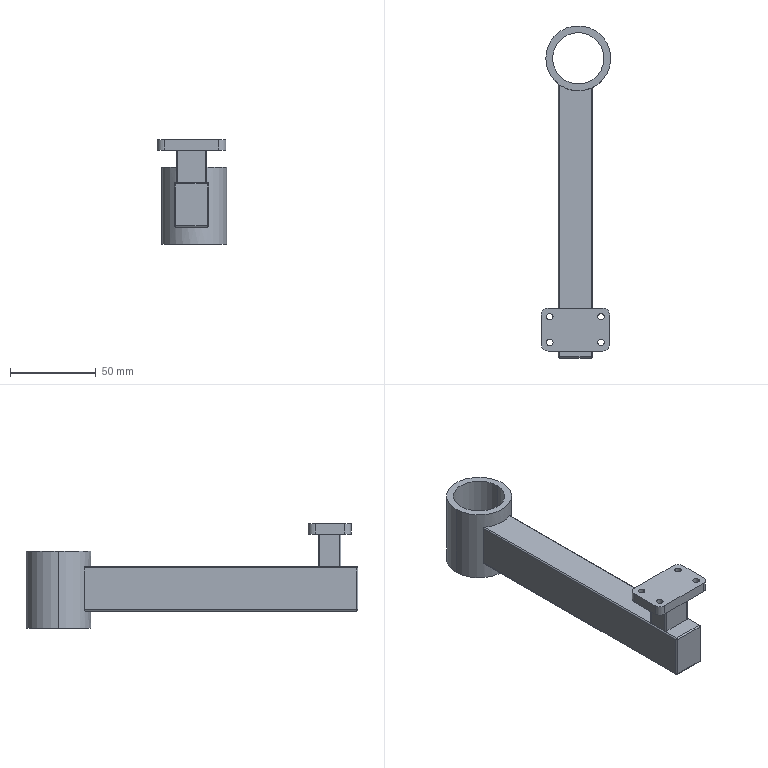Part | SolidWorks | features ICE 3, Extrusion 1, Fillet 1 | 1 solid | 49 faces | box 40.662 x 194 x 61 mm | volume 110850 mm3 | cylinder 28 | plane 17 | sphere 4 | commonest cylinder face diameters 1.6 x12 3.8 x8 8 x4 30 x2 38 x2
STEP:
#1=CARTESIAN_POINT('',(16.662,158.5,-10.));
#2=VERTEX_POINT('',#1);
#3=CARTESIAN_POINT('',(-13.338,158.5,-10.));
#4=VERTEX_POINT('',#3);
#5=CARTESIAN_POINT('',(1.662,158.5,-10.));
#6=DIRECTION('',(0.,0.,-1.));
#7=DIRECTION('',(-1.,0.,0.));
#8=AXIS2_PLACEMENT_3D('',#5,#6,#7);
#9=CIRCLE('',#8,15.);
#10=EDGE_CURVE('',#2,#4,#9,.T.);
#11=ORIENTED_EDGE('',*,*,#10,.F.);
#12=CARTESIAN_POINT('',(16.662,158.5,-55.));
#13=VERTEX_POINT('',#12);
#14=CARTESIAN_POINT('',(16.662,158.5,-10.));
#15=DIRECTION('',(0.,0.,-1.));
#16=VECTOR('',#15,1000.);
#17=LINE('',#14,#16);
#18=EDGE_CURVE('',#2,#13,#17,.T.);
#19=ORIENTED_EDGE('',*,*,#18,.T.);
#20=CARTESIAN_POINT('',(-13.338,158.5,-55.));
#21=VERTEX_POINT('',#20);
#22=CARTESIAN_POINT('',(1.662,158.5,-55.));
#23=DIRECTION('',(0.,0.,-1.));
#24=DIRECTION('',(-1.,0.,0.));
#25=AXIS2_PLACEMENT_3D('',#22,#23,#24);
#26=CIRCLE('',#25,15.);
#27=EDGE_CURVE('',#13,#21,#26,.T.);
#28=ORIENTED_EDGE('',*,*,#27,.T.);
#29=CARTESIAN_POINT('',(-13.338,158.5,-10.));
#30=DIRECTION('',(0.,0.,-1.));
#31=VECTOR('',#30,1000.);
#32=LINE('',#29,#31);
#33=EDGE_CURVE('',#4,#21,#32,.T.);
#34=ORIENTED_EDGE('',*,*,#33,.F.);
#35=EDGE_LOOP('',(#11,#19,#28,#34));
#36=FACE_OUTER_BOUND('',#35,.T.);
#37=CARTESIAN_POINT('',(1.662,158.5,-10.));
#38=DIRECTION('',(0.,0.,-1.));
#39=DIRECTION('',(-1.,0.,0.));
#40=AXIS2_PLACEMENT_3D('',#37,#38,#39);
#41=CYLINDRICAL_SURFACE('',#40,15.);
#42=ADVANCED_FACE('',(#36),#41,.F.);
#43=CARTESIAN_POINT('',(-17.338,158.5,-10.));
#44=VERTEX_POINT('',#43);
#45=CARTESIAN_POINT('',(20.662,158.5,-10.));
#46=VERTEX_POINT('',#45);
#47=CARTESIAN_POINT('',(1.662,158.5,-10.));
#48=DIRECTION('',(0.,0.,-1.));
#49=DIRECTION('',(-1.,0.,0.));
#50=AXIS2_PLACEMENT_3D('',#47,#48,#49);
#51=CIRCLE('',#50,19.);
#52=EDGE_CURVE('',#44,#46,#51,.T.);
#53=ORIENTED_EDGE('',*,*,#52,.T.);
#54=CARTESIAN_POINT('',(20.662,158.5,-55.));
#55=VERTEX_POINT('',#54);
#56=CARTESIAN_POINT('',(20.662,158.5,-10.));
#57=DIRECTION('',(0.,0.,-1.));
#58=VECTOR('',#57,1000.);
#59=LINE('',#56,#58);
#60=EDGE_CURVE('',#46,#55,#59,.T.);
#61=ORIENTED_EDGE('',*,*,#60,.T.);
#62=CARTESIAN_POINT('',(-17.338,158.5,-55.));
#63=VERTEX_POINT('',#62);
#64=CARTESIAN_POINT('',(1.662,158.5,-55.));
#65=DIRECTION('',(0.,0.,-1.));
#66=DIRECTION('',(-1.,0.,0.));
#67=AXIS2_PLACEMENT_3D('',#64,#65,#66);
#68=CIRCLE('',#67,19.);
#69=EDGE_CURVE('',#63,#55,#68,.T.);
#70=ORIENTED_EDGE('',*,*,#69,.F.);
#71=CARTESIAN_POINT('',(-17.338,158.5,-10.));
#72=DIRECTION('',(0.,0.,-1.));
#73=VECTOR('',#72,1000.);
#74=LINE('',#71,#73);
#75=EDGE_CURVE('',#44,#63,#74,.T.);
#76=ORIENTED_EDGE('',*,*,#75,.F.);
#77=EDGE_LOOP('',(#53,#61,#70,#76));
#78=FACE_OUTER_BOUND('',#77,.T.);
#79=CARTESIAN_POINT('',(1.662,158.5,-10.));
#80=DIRECTION('',(0.,0.,-1.));
#81=DIRECTION('',(-1.,0.,0.));
#82=AXIS2_PLACEMENT_3D('',#79,#80,#81);
#83=CYLINDRICAL_SURFACE('',#82,19.);
#84=ADVANCED_FACE('',(#78),#83,.T.);
#85=CARTESIAN_POINT('',(-16.9,-7.5,6.));
#86=VERTEX_POINT('',#85);
#87=CARTESIAN_POINT('',(-13.1,-7.5,6.));
#88=VERTEX_POINT('',#87);
#89=CARTESIAN_POINT('',(-15.,-7.5,6.));
#90=DIRECTION('',(0.,0.,1.));
#91=DIRECTION('',(1.,0.,0.));
#92=AXIS2_PLACEMENT_3D('',#89,#90,#91);
#93=CIRCLE('',#92,1.9);
#94=EDGE_CURVE('',#86,#88,#93,.T.);
#95=ORIENTED_EDGE('',*,*,#94,.T.);
#96=CARTESIAN_POINT('',(-13.1,-7.5,0.));
#97=VERTEX_POINT('',#96);
#98=CARTESIAN_POINT('',(-13.1,-7.5,6.));
#99=DIRECTION('',(0.,0.,-1.));
#100=VECTOR('',#99,1000.);
#101=LINE('',#98,#100);
#102=EDGE_CURVE('',#88,#97,#101,.T.);
#103=ORIENTED_EDGE('',*,*,#102,.T.);
#104=CARTESIAN_POINT('',(-16.9,-7.5,0.));
#105=VERTEX_POINT('',#104);
#106=CARTESIAN_POINT('',(-15.,-7.5,0.));
#107=DIRECTION('',(0.,0.,1.));
#108=DIRECTION('',(1.,0.,0.));
#109=AXIS2_PLACEMENT_3D('',#106,#107,#108);
#110=CIRCLE('',#109,1.9);
#111=EDGE_CURVE('',#105,#97,#110,.T.);
#112=ORIENTED_EDGE('',*,*,#111,.F.);
#113=CARTESIAN_POINT('',(-16.9,-7.5,6.));
#114=DIRECTION('',(0.,0.,-1.));
#115=VECTOR('',#114,1000.);
#116=LINE('',#113,#115);
#117=EDGE_CURVE('',#86,#105,#116,.T.);
#118=ORIENTED_EDGE('',*,*,#117,.F.);
#119=EDGE_LOOP('',(#95,#103,#112,#118));
#120=FACE_OUTER_BOUND('',#119,.T.);
#121=CARTESIAN_POINT('',(-15.,-7.5,6.));
#122=DIRECTION('',(0.,0.,-1.));
#123=DIRECTION('',(-1.,0.,0.));
#124=AXIS2_PLACEMENT_3D('',#121,#122,#123);
#125=CYLINDRICAL_SURFACE('',#124,1.9);
#126=ADVANCED_FACE('',(#120),#125,.F.);
#127=CARTESIAN_POINT('',(13.1,-7.5,6.));
#128=VERTEX_POINT('',#127);
#129=CARTESIAN_POINT('',(16.9,-7.5,6.));
#130=VERTEX_POINT('',#129);
#131=CARTESIAN_POINT('',(15.,-7.5,6.));
#132=DIRECTION('',(0.,0.,1.));
#133=DIRECTION('',(1.,0.,0.));
#134=AXIS2_PLACEMENT_3D('',#131,#132,#133);
#135=CIRCLE('',#134,1.9);
#136=EDGE_CURVE('',#128,#130,#135,.T.);
#137=ORIENTED_EDGE('',*,*,#136,.T.);
#138=CARTESIAN_POINT('',(16.9,-7.5,0.));
#139=VERTEX_POINT('',#138);
#140=CARTESIAN_POINT('',(16.9,-7.5,6.));
#141=DIRECTION('',(0.,0.,-1.));
#142=VECTOR('',#141,1000.);
#143=LINE('',#140,#142);
#144=EDGE_CURVE('',#130,#139,#143,.T.);
#145=ORIENTED_EDGE('',*,*,#144,.T.);
#146=CARTESIAN_POINT('',(13.1,-7.5,0.));
#147=VERTEX_POINT('',#146);
#148=CARTESIAN_POINT('',(15.,-7.5,0.));
#149=DIRECTION('',(0.,0.,1.));
#150=DIRECTION('',(1.,0.,0.));
#151=AXIS2_PLACEMENT_3D('',#148,#149,#150);
#152=CIRCLE('',#151,1.9);
#153=EDGE_CURVE('',#147,#139,#152,.T.);
#154=ORIENTED_EDGE('',*,*,#153,.F.);
#155=CARTESIAN_POINT('',(13.1,-7.5,6.));
#156=DIRECTION('',(0.,0.,-1.));
#157=VECTOR('',#156,1000.);
#158=LINE('',#155,#157);
#159=EDGE_CURVE('',#128,#147,#158,.T.);
#160=ORIENTED_EDGE('',*,*,#159,.F.);
#161=EDGE_LOOP('',(#137,#145,#154,#160));
#162=FACE_OUTER_BOUND('',#161,.T.);
#163=CARTESIAN_POINT('',(15.,-7.5,6.));
#164=DIRECTION('',(0.,0.,-1.));
#165=DIRECTION('',(-1.,0.,0.));
#166=AXIS2_PLACEMENT_3D('',#163,#164,#165);
#167=CYLINDRICAL_SURFACE('',#166,1.9);
#168=ADVANCED_FACE('',(#162),#167,.F.);
#169=CARTESIAN_POINT('',(13.1,7.5,6.));
#170=VERTEX_POINT('',#169);
#171=CARTESIAN_POINT('',(16.9,7.5,6.));
#172=VERTEX_POINT('',#171);
#173=CARTESIAN_POINT('',(15.,7.5,6.));
#174=DIRECTION('',(0.,0.,1.));
#175=DIRECTION('',(1.,0.,0.));
#176=AXIS2_PLACEMENT_3D('',#173,#174,#175);
#177=CIRCLE('',#176,1.9);
#178=EDGE_CURVE('',#170,#172,#177,.T.);
#179=ORIENTED_EDGE('',*,*,#178,.T.);
#180=CARTESIAN_POINT('',(16.9,7.5,0.));
#181=VERTEX_POINT('',#180);
#182=CARTESIAN_POINT('',(16.9,7.5,6.));
#183=DIRECTION('',(0.,0.,-1.));
#184=VECTOR('',#183,1000.);
#185=LINE('',#182,#184);
#186=EDGE_CURVE('',#172,#181,#185,.T.);
#187=ORIENTED_EDGE('',*,*,#186,.T.);
#188=CARTESIAN_POINT('',(13.1,7.5,0.));
#189=VERTEX_POINT('',#188);
#190=CARTESIAN_POINT('',(15.,7.5,0.));
#191=DIRECTION('',(0.,0.,1.));
#192=DIRECTION('',(1.,0.,0.));
#193=AXIS2_PLACEMENT_3D('',#190,#191,#192);
#194=CIRCLE('',#193,1.9);
#195=EDGE_CURVE('',#189,#181,#194,.T.);
#196=ORIENTED_EDGE('',*,*,#195,.F.);
#197=CARTESIAN_POINT('',(13.1,7.5,6.));
#198=DIRECTION('',(0.,0.,-1.));
#199=VECTOR('',#198,1000.);
#200=LINE('',#197,#199);
#201=EDGE_CURVE('',#170,#189,#200,.T.);
#202=ORIENTED_EDGE('',*,*,#201,.F.);
#203=EDGE_LOOP('',(#179,#187,#196,#202));
#204=FACE_OUTER_BOUND('',#203,.T.);
#205=CARTESIAN_POINT('',(15.,7.5,6.));
#206=DIRECTION('',(0.,0.,-1.));
#207=DIRECTION('',(-1.,0.,0.));
#208=AXIS2_PLACEMENT_3D('',#205,#206,#207);
#209=CYLINDRICAL_SURFACE('',#208,1.9);
#210=ADVANCED_FACE('',(#204),#209,.F.);
#211=CARTESIAN_POINT('',(-16.9,7.5,6.));
#212=VERTEX_POINT('',#211);
#213=CARTESIAN_POINT('',(-13.1,7.5,6.));
#214=VERTEX_POINT('',#213);
#215=CARTESIAN_POINT('',(-15.,7.5,6.));
#216=DIRECTION('',(0.,0.,1.));
#217=DIRECTION('',(1.,0.,0.));
#218=AXIS2_PLACEMENT_3D('',#215,#216,#217);
#219=CIRCLE('',#218,1.9);
#220=EDGE_CURVE('',#212,#214,#219,.T.);
#221=ORIENTED_EDGE('',*,*,#220,.T.);
#222=CARTESIAN_POINT('',(-13.1,7.5,0.));
#223=VERTEX_POINT('',#222);
#224=CARTESIAN_POINT('',(-13.1,7.5,6.));
#225=DIRECTION('',(0.,0.,-1.));
#226=VECTOR('',#225,1000.);
#227=LINE('',#224,#226);
#228=EDGE_CURVE('',#214,#223,#227,.T.);
#229=ORIENTED_EDGE('',*,*,#228,.T.);
#230=CARTESIAN_POINT('',(-16.9,7.5,0.));
#231=VERTEX_POINT('',#230);
#232=CARTESIAN_POINT('',(-15.,7.5,0.));
#233=DIRECTION('',(0.,0.,1.));
#234=DIRECTION('',(1.,0.,0.));
#235=AXIS2_PLACEMENT_3D('',#232,#233,#234);
#236=CIRCLE('',#235,1.9);
#237=EDGE_CURVE('',#231,#223,#236,.T.);
#238=ORIENTED_EDGE('',*,*,#237,.F.);
#239=CARTESIAN_POINT('',(-16.9,7.5,6.));
#240=DIRECTION('',(0.,0.,-1.));
#241=VECTOR('',#240,1000.);
#242=LINE('',#239,#241);
#243=EDGE_CURVE('',#212,#231,#242,.T.);
#244=ORIENTED_EDGE('',*,*,#243,.F.);
#245=EDGE_LOOP('',(#221,#229,#238,#244));
#246=FACE_OUTER_BOUND('',#245,.T.);
#247=CARTESIAN_POINT('',(-15.,7.5,6.));
#248=DIRECTION('',(0.,0.,-1.));
#249=DIRECTION('',(-1.,0.,0.));
#250=AXIS2_PLACEMENT_3D('',#247,#248,#249);
#251=CYLINDRICAL_SURFACE('',#250,1.9);
#252=ADVANCED_FACE('',(#246),#251,.F.);
#253=ORIENTED_EDGE('',*,*,#111,.T.);
#254=CARTESIAN_POINT('',(-15.,-7.5,0.));
#255=DIRECTION('',(0.,0.,1.));
#256=DIRECTION('',(1.,0.,0.));
#257=AXIS2_PLACEMENT_3D('',#254,#255,#256);
#258=CIRCLE('',#257,1.9);
#259=EDGE_CURVE('',#97,#105,#258,.T.);
#260=ORIENTED_EDGE('',*,*,#259,.T.);
#261=EDGE_LOOP('',(#253,#260));
#262=FACE_BOUND('',#261,.T.);
#263=ORIENTED_EDGE('',*,*,#153,.T.);
#264=CARTESIAN_POINT('',(15.,-7.5,0.));
#265=DIRECTION('',(0.,0.,1.));
#266=DIRECTION('',(1.,0.,0.));
#267=AXIS2_PLACEMENT_3D('',#264,#265,#266);
#268=CIRCLE('',#267,1.9);
#269=EDGE_CURVE('',#139,#147,#268,.T.);
#270=ORIENTED_EDGE('',*,*,#269,.T.);
#271=EDGE_LOOP('',(#263,#270));
#272=FACE_BOUND('',#271,.T.);
#273=ORIENTED_EDGE('',*,*,#195,.T.);
#274=CARTESIAN_POINT('',(15.,7.5,0.));
#275=DIRECTION('',(0.,0.,1.));
#276=DIRECTION('',(1.,0.,0.));
#277=AXIS2_PLACEMENT_3D('',#274,#275,#276);
#278=CIRCLE('',#277,1.9);
#279=EDGE_CURVE('',#181,#189,#278,.T.);
#280=ORIENTED_EDGE('',*,*,#279,.T.);
#281=EDGE_LOOP('',(#273,#280));
#282=FACE_BOUND('',#281,.T.);
#283=ORIENTED_EDGE('',*,*,#237,.T.);
#284=CARTESIAN_POINT('',(-15.,7.5,0.));
#285=DIRECTION('',(0.,0.,1.));
#286=DIRECTION('',(1.,0.,0.));
#287=AXIS2_PLACEMENT_3D('',#284,#285,#286);
#288=CIRCLE('',#287,1.9);
#289=EDGE_CURVE('',#223,#231,#288,.T.);
#290=ORIENTED_EDGE('',*,*,#289,.T.);
#291=EDGE_LOOP('',(#283,#290));
#292=FACE_BOUND('',#291,.T.);
#293=CARTESIAN_POINT('',(-20.,-8.5,0.));
#294=VERTEX_POINT('',#293);
#295=CARTESIAN_POINT('',(-16.,-12.5,0.));
#296=VERTEX_POINT('',#295);
#297=CARTESIAN_POINT('',(-16.,-8.5,0.));
#298=DIRECTION('',(0.,0.,1.));
#299=DIRECTION('',(1.,0.,0.));
#300=AXIS2_PLACEMENT_3D('',#297,#298,#299);
#301=CIRCLE('',#300,4.);
#302=EDGE_CURVE('',#294,#296,#301,.T.);
#303=ORIENTED_EDGE('',*,*,#302,.F.);
#304=CARTESIAN_POINT('',(-20.,8.5,0.));
#305=VERTEX_POINT('',#304);
#306=CARTESIAN_POINT('',(-20.,8.5,0.));
#307=DIRECTION('',(0.,-1.,0.));
#308=VECTOR('',#307,1000.);
#309=LINE('',#306,#308);
#310=EDGE_CURVE('',#305,#294,#309,.T.);
#311=ORIENTED_EDGE('',*,*,#310,.F.);
#312=CARTESIAN_POINT('',(-16.,12.5,0.));
#313=VERTEX_POINT('',#312);
#314=CARTESIAN_POINT('',(-16.,8.5,0.));
#315=DIRECTION('',(0.,0.,1.));
#316=DIRECTION('',(1.,0.,0.));
#317=AXIS2_PLACEMENT_3D('',#314,#315,#316);
#318=CIRCLE('',#317,4.);
#319=EDGE_CURVE('',#313,#305,#318,.T.);
#320=ORIENTED_EDGE('',*,*,#319,.F.);
#321=CARTESIAN_POINT('',(16.,12.5,0.));
#322=VERTEX_POINT('',#321);
#323=CARTESIAN_POINT('',(-16.,12.5,0.));
#324=DIRECTION('',(-1.,0.,0.));
#325=VECTOR('',#324,1000.);
#326=LINE('',#323,#325);
#327=EDGE_CURVE('',#322,#313,#326,.T.);
#328=ORIENTED_EDGE('',*,*,#327,.F.);
#329=CARTESIAN_POINT('',(20.,8.5,0.));
#330=VERTEX_POINT('',#329);
#331=CARTESIAN_POINT('',(16.,8.5,0.));
#332=DIRECTION('',(0.,0.,1.));
#333=DIRECTION('',(-1.,0.,0.));
#334=AXIS2_PLACEMENT_3D('',#331,#332,#333);
#335=CIRCLE('',#334,4.);
#336=EDGE_CURVE('',#330,#322,#335,.T.);
#337=ORIENTED_EDGE('',*,*,#336,.F.);
#338=CARTESIAN_POINT('',(20.,-8.5,0.));
#339=VERTEX_POINT('',#338);
#340=CARTESIAN_POINT('',(20.,8.5,0.));
#341=DIRECTION('',(0.,1.,0.));
#342=VECTOR('',#341,1000.);
#343=LINE('',#340,#342);
#344=EDGE_CURVE('',#339,#330,#343,.T.);
#345=ORIENTED_EDGE('',*,*,#344,.F.);
#346=CARTESIAN_POINT('',(16.,-12.5,0.));
#347=VERTEX_POINT('',#346);
#348=CARTESIAN_POINT('',(16.,-8.5,0.));
#349=DIRECTION('',(0.,0.,1.));
#350=DIRECTION('',(1.,0.,0.));
#351=AXIS2_PLACEMENT_3D('',#348,#349,#350);
#352=CIRCLE('',#351,4.);
#353=EDGE_CURVE('',#347,#339,#352,.T.);
#354=ORIENTED_EDGE('',*,*,#353,.F.);
#355=CARTESIAN_POINT('',(-16.,-12.5,0.));
#356=DIRECTION('',(1.,0.,0.));
#357=VECTOR('',#356,1000.);
#358=LINE('',#355,#357);
#359=EDGE_CURVE('',#296,#347,#358,.T.);
#360=ORIENTED_EDGE('',*,*,#359,.F.);
#361=EDGE_LOOP('',(#303,#311,#320,#328,#337,#345,#354,#360));
#362=FACE_OUTER_BOUND('',#361,.T.);
#363=CARTESIAN_POINT('',(-9.,-5.7,0.));
#364=VERTEX_POINT('',#363);
#365=CARTESIAN_POINT('',(-9.,5.7,0.));
#366=VERTEX_POINT('',#365);
#367=CARTESIAN_POINT('',(-9.,6.5,0.));
#368=DIRECTION('',(0.,1.,0.));
#369=VECTOR('',#368,1000.);
#370=LINE('',#367,#369);
#371=EDGE_CURVE('',#364,#366,#370,.T.);
#372=ORIENTED_EDGE('',*,*,#371,.F.);
#373=CARTESIAN_POINT('',(-8.2,-6.5,0.));
#374=VERTEX_POINT('',#373);
#375=CARTESIAN_POINT('',(-8.2,-5.7,0.));
#376=DIRECTION('',(0.,0.,1.));
#377=DIRECTION('',(1.,0.,0.));
#378=AXIS2_PLACEMENT_3D('',#375,#376,#377);
#379=CIRCLE('',#378,0.8);
#380=EDGE_CURVE('',#364,#374,#379,.T.);
#381=ORIENTED_EDGE('',*,*,#380,.T.);
#382=CARTESIAN_POINT('',(8.2,-6.5,0.));
#383=VERTEX_POINT('',#382);
#384=CARTESIAN_POINT('',(9.,-6.5,0.));
#385=DIRECTION('',(-1.,0.,0.));
#386=VECTOR('',#385,1000.);
#387=LINE('',#384,#386);
#388=EDGE_CURVE('',#383,#374,#387,.T.);
#389=ORIENTED_EDGE('',*,*,#388,.F.);
#390=CARTESIAN_POINT('',(9.,-5.7,0.));
#391=VERTEX_POINT('',#390);
#392=CARTESIAN_POINT('',(8.2,-5.7,0.));
#393=DIRECTION('',(0.,0.,1.));
#394=DIRECTION('',(1.,0.,0.));
#395=AXIS2_PLACEMENT_3D('',#392,#393,#394);
#396=CIRCLE('',#395,0.8);
#397=EDGE_CURVE('',#383,#391,#396,.T.);
#398=ORIENTED_EDGE('',*,*,#397,.T.);
#399=CARTESIAN_POINT('',(9.,5.7,0.));
#400=VERTEX_POINT('',#399);
#401=CARTESIAN_POINT('',(9.,6.5,0.));
#402=DIRECTION('',(0.,-1.,0.));
#403=VECTOR('',#402,1000.);
#404=LINE('',#401,#403);
#405=EDGE_CURVE('',#400,#391,#404,.T.);
#406=ORIENTED_EDGE('',*,*,#405,.F.);
#407=CARTESIAN_POINT('',(8.2,6.5,0.));
#408=VERTEX_POINT('',#407);
#409=CARTESIAN_POINT('',(8.2,5.7,0.));
#410=DIRECTION('',(0.,0.,1.));
#411=DIRECTION('',(1.,0.,0.));
#412=AXIS2_PLACEMENT_3D('',#409,#410,#411);
#413=CIRCLE('',#412,0.8);
#414=EDGE_CURVE('',#400,#408,#413,.T.);
#415=ORIENTED_EDGE('',*,*,#414,.T.);
#416=CARTESIAN_POINT('',(-8.2,6.5,0.));
#417=VERTEX_POINT('',#416);
#418=CARTESIAN_POINT('',(9.,6.5,0.));
#419=DIRECTION('',(1.,0.,0.));
#420=VECTOR('',#419,1000.);
#421=LINE('',#418,#420);
#422=EDGE_CURVE('',#417,#408,#421,.T.);
#423=ORIENTED_EDGE('',*,*,#422,.F.);
#424=CARTESIAN_POINT('',(-8.2,5.7,0.));
#425=DIRECTION('',(0.,0.,1.));
#426=DIRECTION('',(1.,0.,0.));
#427=AXIS2_PLACEMENT_3D('',#424,#425,#426);
#428=CIRCLE('',#427,0.8);
#429=EDGE_CURVE('',#417,#366,#428,.T.);
#430=ORIENTED_EDGE('',*,*,#429,.T.);
#431=EDGE_LOOP('',(#372,#381,#389,#398,#406,#415,#423,#430));
#432=FACE_BOUND('',#431,.T.);
#433=CARTESIAN_POINT('',(-16.,-8.5,0.));
#434=DIRECTION('',(0.,0.,1.));
#435=DIRECTION('',(1.,0.,0.));
#436=AXIS2_PLACEMENT_3D('',#433,#434,#435);
#437=PLANE('',#436);
#438=ADVANCED_FACE('',(#262,#272,#282,#292,#362,#432),#437,.F.);
#439=ORIENTED_EDGE('',*,*,#136,.F.);
#440=CARTESIAN_POINT('',(15.,-7.5,6.));
#441=DIRECTION('',(0.,0.,1.));
#442=DIRECTION('',(1.,0.,0.));
#443=AXIS2_PLACEMENT_3D('',#440,#441,#442);
#444=CIRCLE('',#443,1.9);
#445=EDGE_CURVE('',#130,#128,#444,.T.);
#446=ORIENTED_EDGE('',*,*,#445,.F.);
#447=EDGE_LOOP('',(#439,#446));
#448=FACE_BOUND('',#447,.T.);
#449=ORIENTED_EDGE('',*,*,#220,.F.);
#450=CARTESIAN_POINT('',(-15.,7.5,6.));
#451=DIRECTION('',(0.,0.,1.));
#452=DIRECTION('',(1.,0.,0.));
#453=AXIS2_PLACEMENT_3D('',#450,#451,#452);
#454=CIRCLE('',#453,1.9);
#455=EDGE_CURVE('',#214,#212,#454,.T.);
#456=ORIENTED_EDGE('',*,*,#455,.F.);
#457=EDGE_LOOP('',(#449,#456));
#458=FACE_BOUND('',#457,.T.);
#459=CARTESIAN_POINT('',(-20.,-8.5,6.));
#460=VERTEX_POINT('',#459);
#461=CARTESIAN_POINT('',(-16.,-12.5,6.));
#462=VERTEX_POINT('',#461);
#463=CARTESIAN_POINT('',(-16.,-8.5,6.));
#464=DIRECTION('',(0.,0.,1.));
#465=DIRECTION('',(1.,0.,0.));
#466=AXIS2_PLACEMENT_3D('',#463,#464,#465);
#467=CIRCLE('',#466,4.);
#468=EDGE_CURVE('',#460,#462,#467,.T.);
#469=ORIENTED_EDGE('',*,*,#468,.T.);
#470=CARTESIAN_POINT('',(16.,-12.5,6.));
#471=VERTEX_POINT('',#470);
#472=CARTESIAN_POINT('',(-16.,-12.5,6.));
#473=DIRECTION('',(1.,0.,0.));
#474=VECTOR('',#473,1000.);
#475=LINE('',#472,#474);
#476=EDGE_CURVE('',#462,#471,#475,.T.);
#477=ORIENTED_EDGE('',*,*,#476,.T.);
#478=CARTESIAN_POINT('',(20.,-8.5,6.));
#479=VERTEX_POINT('',#478);
#480=CARTESIAN_POINT('',(16.,-8.5,6.));
#481=DIRECTION('',(0.,0.,1.));
#482=DIRECTION('',(1.,0.,0.));
#483=AXIS2_PLACEMENT_3D('',#480,#481,#482);
#484=CIRCLE('',#483,4.);
#485=EDGE_CURVE('',#471,#479,#484,.T.);
#486=ORIENTED_EDGE('',*,*,#485,.T.);
#487=CARTESIAN_POINT('',(20.,8.5,6.));
#488=VERTEX_POINT('',#487);
#489=CARTESIAN_POINT('',(20.,8.5,6.));
#490=DIRECTION('',(0.,1.,0.));
#491=VECTOR('',#490,1000.);
#492=LINE('',#489,#491);
#493=EDGE_CURVE('',#479,#488,#492,.T.);
#494=ORIENTED_EDGE('',*,*,#493,.T.);
#495=CARTESIAN_POINT('',(16.,12.5,6.));
#496=VERTEX_POINT('',#495);
#497=CARTESIAN_POINT('',(16.,8.5,6.));
#498=DIRECTION('',(0.,0.,1.));
#499=DIRECTION('',(-1.,0.,0.));
#500=AXIS2_PLACEMENT_3D('',#497,#498,#499);
#501=CIRCLE('',#500,4.);
#502=EDGE_CURVE('',#488,#496,#501,.T.);
#503=ORIENTED_EDGE('',*,*,#502,.T.);
#504=CARTESIAN_POINT('',(-16.,12.5,6.));
#505=VERTEX_POINT('',#504);
#506=CARTESIAN_POINT('',(-16.,12.5,6.));
#507=DIRECTION('',(-1.,0.,0.));
#508=VECTOR('',#507,1000.);
#509=LINE('',#506,#508);
#510=EDGE_CURVE('',#496,#505,#509,.T.);
#511=ORIENTED_EDGE('',*,*,#510,.T.);
#512=CARTESIAN_POINT('',(-20.,8.5,6.));
#513=VERTEX_POINT('',#512);
#514=CARTESIAN_POINT('',(-16.,8.5,6.));
#515=DIRECTION('',(0.,0.,1.));
#516=DIRECTION('',(1.,0.,0.));
#517=AXIS2_PLACEMENT_3D('',#514,#515,#516);
#518=CIRCLE('',#517,4.);
#519=EDGE_CURVE('',#505,#513,#518,.T.);
#520=ORIENTED_EDGE('',*,*,#519,.T.);
#521=CARTESIAN_POINT('',(-20.,8.5,6.));
#522=DIRECTION('',(0.,-1.,0.));
#523=VECTOR('',#522,1000.);
#524=LINE('',#521,#523);
#525=EDGE_CURVE('',#513,#460,#524,.T.);
#526=ORIENTED_EDGE('',*,*,#525,.T.);
#527=EDGE_LOOP('',(#469,#477,#486,#494,#503,#511,#520,#526));
#528=FACE_OUTER_BOUND('',#527,.T.);
#529=ORIENTED_EDGE('',*,*,#178,.F.);
#530=CARTESIAN_POINT('',(15.,7.5,6.));
#531=DIRECTION('',(0.,0.,1.));
#532=DIRECTION('',(1.,0.,0.));
#533=AXIS2_PLACEMENT_3D('',#530,#531,#532);
#534=CIRCLE('',#533,1.9);
#535=EDGE_CURVE('',#172,#170,#534,.T.);
#536=ORIENTED_EDGE('',*,*,#535,.F.);
#537=EDGE_LOOP('',(#529,#536));
#538=FACE_BOUND('',#537,.T.);
#539=ORIENTED_EDGE('',*,*,#94,.F.);
#540=CARTESIAN_POINT('',(-15.,-7.5,6.));
#541=DIRECTION('',(0.,0.,1.));
#542=DIRECTION('',(1.,0.,0.));
#543=AXIS2_PLACEMENT_3D('',#540,#541,#542);
#544=CIRCLE('',#543,1.9);
#545=EDGE_CURVE('',#88,#86,#544,.T.);
#546=ORIENTED_EDGE('',*,*,#545,.F.);
#547=EDGE_LOOP('',(#539,#546));
#548=FACE_BOUND('',#547,.T.);
#549=CARTESIAN_POINT('',(-16.,-8.5,6.));
#550=DIRECTION('',(0.,0.,1.));
#551=DIRECTION('',(1.,0.,0.));
#552=AXIS2_PLACEMENT_3D('',#549,#550,#551);
#553=PLANE('',#552);
#554=ADVANCED_FACE('',(#448,#458,#528,#538,#548),#553,.T.);
#555=ORIENTED_EDGE('',*,*,#302,.T.);
#556=CARTESIAN_POINT('',(-16.,-12.5,6.));
#557=DIRECTION('',(0.,0.,-1.));
#558=VECTOR('',#557,1000.);
#559=LINE('',#556,#558);
#560=EDGE_CURVE('',#462,#296,#559,.T.);
#561=ORIENTED_EDGE('',*,*,#560,.F.);
#562=ORIENTED_EDGE('',*,*,#468,.F.);
#563=CARTESIAN_POINT('',(-20.,-8.5,6.));
#564=DIRECTION('',(0.,0.,-1.));
#565=VECTOR('',#564,1000.);
#566=LINE('',#563,#565);
#567=EDGE_CURVE('',#460,#294,#566,.T.);
#568=ORIENTED_EDGE('',*,*,#567,.T.);
#569=EDGE_LOOP('',(#555,#561,#562,#568));
#570=FACE_OUTER_BOUND('',#569,.T.);
#571=CARTESIAN_POINT('',(-16.,-8.5,6.));
#572=DIRECTION('',(0.,0.,-1.));
#573=DIRECTION('',(-1.,0.,0.));
#574=AXIS2_PLACEMENT_3D('',#571,#572,#573);
#575=CYLINDRICAL_SURFACE('',#574,4.);
#576=ADVANCED_FACE('',(#570),#575,.T.);
#577=ORIENTED_EDGE('',*,*,#359,.T.);
#578=CARTESIAN_POINT('',(16.,-12.5,6.));
#579=DIRECTION('',(0.,0.,-1.));
#580=VECTOR('',#579,1000.);
#581=LINE('',#578,#580);
#582=EDGE_CURVE('',#471,#347,#581,.T.);
#583=ORIENTED_EDGE('',*,*,#582,.F.);
#584=ORIENTED_EDGE('',*,*,#476,.F.);
#585=ORIENTED_EDGE('',*,*,#560,.T.);
#586=EDGE_LOOP('',(#577,#583,#584,#585));
#587=FACE_OUTER_BOUND('',#586,.T.);
#588=CARTESIAN_POINT('',(-16.,-12.5,6.));
#589=DIRECTION('',(0.,1.,0.));
#590=DIRECTION('',(-1.,0.,0.));
#591=AXIS2_PLACEMENT_3D('',#588,#589,#590);
#592=PLANE('',#591);
#593=ADVANCED_FACE('',(#587),#592,.F.);
#594=ORIENTED_EDGE('',*,*,#353,.T.);
#595=CARTESIAN_POINT('',(20.,-8.5,6.));
#596=DIRECTION('',(0.,0.,-1.));
#597=VECTOR('',#596,1000.);
#598=LINE('',#595,#597);
#599=EDGE_CURVE('',#479,#339,#598,.T.);
#600=ORIENTED_EDGE('',*,*,#599,.F.);
#601=ORIENTED_EDGE('',*,*,#485,.F.);
#602=ORIENTED_EDGE('',*,*,#582,.T.);
#603=EDGE_LOOP('',(#594,#600,#601,#602));
#604=FACE_OUTER_BOUND('',#603,.T.);
#605=CARTESIAN_POINT('',(16.,-8.5,6.));
#606=DIRECTION('',(0.,0.,-1.));
#607=DIRECTION('',(-1.,0.,0.));
#608=AXIS2_PLACEMENT_3D('',#605,#606,#607);
#609=CYLINDRICAL_SURFACE('',#608,4.);
#610=ADVANCED_FACE('',(#604),#609,.T.);
#611=ORIENTED_EDGE('',*,*,#344,.T.);
#612=CARTESIAN_POINT('',(20.,8.5,6.));
#613=DIRECTION('',(0.,0.,-1.));
#614=VECTOR('',#613,1000.);
#615=LINE('',#612,#614);
#616=EDGE_CURVE('',#488,#330,#615,.T.);
#617=ORIENTED_EDGE('',*,*,#616,.F.);
#618=ORIENTED_EDGE('',*,*,#493,.F.);
#619=ORIENTED_EDGE('',*,*,#599,.T.);
#620=EDGE_LOOP('',(#611,#617,#618,#619));
#621=FACE_OUTER_BOUND('',#620,.T.);
#622=CARTESIAN_POINT('',(20.,8.5,6.));
#623=DIRECTION('',(-1.,0.,0.));
#624=DIRECTION('',(0.,-1.,0.));
#625=AXIS2_PLACEMENT_3D('',#622,#623,#624);
#626=PLANE('',#625);
#627=ADVANCED_FACE('',(#621),#626,.F.);
#628=ORIENTED_EDGE('',*,*,#336,.T.);
#629=CARTESIAN_POINT('',(16.,12.5,6.));
#630=DIRECTION('',(0.,0.,-1.));
#631=VECTOR('',#630,1000.);
#632=LINE('',#629,#631);
#633=EDGE_CURVE('',#496,#322,#632,.T.);
#634=ORIENTED_EDGE('',*,*,#633,.F.);
#635=ORIENTED_EDGE('',*,*,#502,.F.);
#636=ORIENTED_EDGE('',*,*,#616,.T.);
#637=EDGE_LOOP('',(#628,#634,#635,#636));
#638=FACE_OUTER_BOUND('',#637,.T.);
#639=CARTESIAN_POINT('',(16.,8.5,6.));
#640=DIRECTION('',(0.,0.,-1.));
#641=DIRECTION('',(-1.,0.,0.));
#642=AXIS2_PLACEMENT_3D('',#639,#640,#641);
#643=CYLINDRICAL_SURFACE('',#642,4.);
#644=ADVANCED_FACE('',(#638),#643,.T.);
#645=ORIENTED_EDGE('',*,*,#327,.T.);
#646=CARTESIAN_POINT('',(-16.,12.5,6.));
#647=DIRECTION('',(0.,0.,-1.));
#648=VECTOR('',#647,1000.);
#649=LINE('',#646,#648);
#650=EDGE_CURVE('',#505,#313,#649,.T.);
#651=ORIENTED_EDGE('',*,*,#650,.F.);
#652=ORIENTED_EDGE('',*,*,#510,.F.);
#653=ORIENTED_EDGE('',*,*,#633,.T.);
#654=EDGE_LOOP('',(#645,#651,#652,#653));
#655=FACE_OUTER_BOUND('',#654,.T.);
#656=CARTESIAN_POINT('',(-16.,12.5,6.));
#657=DIRECTION('',(0.,-1.,0.));
#658=DIRECTION('',(0.,0.,-1.));
#659=AXIS2_PLACEMENT_3D('',#656,#657,#658);
#660=PLANE('',#659);
#661=ADVANCED_FACE('',(#655),#660,.F.);
#662=ORIENTED_EDGE('',*,*,#319,.T.);
#663=CARTESIAN_POINT('',(-20.,8.5,6.));
#664=DIRECTION('',(0.,0.,-1.));
#665=VECTOR('',#664,1000.);
#666=LINE('',#663,#665);
#667=EDGE_CURVE('',#513,#305,#666,.T.);
#668=ORIENTED_EDGE('',*,*,#667,.F.);
#669=ORIENTED_EDGE('',*,*,#519,.F.);
#670=ORIENTED_EDGE('',*,*,#650,.T.);
#671=EDGE_LOOP('',(#662,#668,#669,#670));
#672=FACE_OUTER_BOUND('',#671,.T.);
#673=CARTESIAN_POINT('',(-16.,8.5,6.));
#674=DIRECTION('',(0.,0.,-1.));
#675=DIRECTION('',(-1.,0.,0.));
#676=AXIS2_PLACEMENT_3D('',#673,#674,#675);
#677=CYLINDRICAL_SURFACE('',#676,4.);
#678=ADVANCED_FACE('',(#672),#677,.T.);
#679=ORIENTED_EDGE('',*,*,#310,.T.);
#680=ORIENTED_EDGE('',*,*,#567,.F.);
#681=ORIENTED_EDGE('',*,*,#525,.F.);
#682=ORIENTED_EDGE('',*,*,#667,.T.);
#683=EDGE_LOOP('',(#679,#680,#681,#682));
#684=FACE_OUTER_BOUND('',#683,.T.);
#685=CARTESIAN_POINT('',(-20.,8.5,6.));
#686=DIRECTION('',(1.,0.,0.));
#687=DIRECTION('',(0.,1.,0.));
#688=AXIS2_PLACEMENT_3D('',#685,#686,#687);
#689=PLANE('',#688);
#690=ADVANCED_FACE('',(#684),#689,.F.);
#691=ORIENTED_EDGE('',*,*,#228,.F.);
#692=ORIENTED_EDGE('',*,*,#455,.T.);
#693=ORIENTED_EDGE('',*,*,#243,.T.);
#694=ORIENTED_EDGE('',*,*,#289,.F.);
#695=EDGE_LOOP('',(#691,#692,#693,#694));
#696=FACE_OUTER_BOUND('',#695,.T.);
#697=CARTESIAN_POINT('',(-15.,7.5,6.));
#698=DIRECTION('',(0.,0.,-1.));
#699=DIRECTION('',(-1.,0.,0.));
#700=AXIS2_PLACEMENT_3D('',#697,#698,#699);
#701=CYLINDRICAL_SURFACE('',#700,1.9);
#702=ADVANCED_FACE('',(#696),#701,.F.);
#703=ORIENTED_EDGE('',*,*,#186,.F.);
#704=ORIENTED_EDGE('',*,*,#535,.T.);
#705=ORIENTED_EDGE('',*,*,#201,.T.);
#706=ORIENTED_EDGE('',*,*,#279,.F.);
#707=EDGE_LOOP('',(#703,#704,#705,#706));
#708=FACE_OUTER_BOUND('',#707,.T.);
#709=CARTESIAN_POINT('',(15.,7.5,6.));
#710=DIRECTION('',(0.,0.,-1.));
#711=DIRECTION('',(-1.,0.,0.));
#712=AXIS2_PLACEMENT_3D('',#709,#710,#711);
#713=CYLINDRICAL_SURFACE('',#712,1.9);
#714=ADVANCED_FACE('',(#708),#713,.F.);
#715=ORIENTED_EDGE('',*,*,#144,.F.);
#716=ORIENTED_EDGE('',*,*,#445,.T.);
#717=ORIENTED_EDGE('',*,*,#159,.T.);
#718=ORIENTED_EDGE('',*,*,#269,.F.);
#719=EDGE_LOOP('',(#715,#716,#717,#718));
#720=FACE_OUTER_BOUND('',#719,.T.);
#721=CARTESIAN_POINT('',(15.,-7.5,6.));
#722=DIRECTION('',(0.,0.,-1.));
#723=DIRECTION('',(-1.,0.,0.));
#724=AXIS2_PLACEMENT_3D('',#721,#722,#723);
#725=CYLINDRICAL_SURFACE('',#724,1.9);
#726=ADVANCED_FACE('',(#720),#725,.F.);
#727=ORIENTED_EDGE('',*,*,#102,.F.);
#728=ORIENTED_EDGE('',*,*,#545,.T.);
#729=ORIENTED_EDGE('',*,*,#117,.T.);
#730=ORIENTED_EDGE('',*,*,#259,.F.);
#731=EDGE_LOOP('',(#727,#728,#729,#730));
#732=FACE_OUTER_BOUND('',#731,.T.);
#733=CARTESIAN_POINT('',(-15.,-7.5,6.));
#734=DIRECTION('',(0.,0.,-1.));
#735=DIRECTION('',(-1.,0.,0.));
#736=AXIS2_PLACEMENT_3D('',#733,#734,#735);
#737=CYLINDRICAL_SURFACE('',#736,1.9);
#738=ADVANCED_FACE('',(#732),#737,.F.);
#739=CARTESIAN_POINT('',(-9.,5.7,-19.));
#740=VERTEX_POINT('',#739);
#741=CARTESIAN_POINT('',(-9.,-5.7,-19.));
#742=VERTEX_POINT('',#741);
#743=CARTESIAN_POINT('',(-9.,6.5,-19.));
#744=DIRECTION('',(0.,-1.,0.));
#745=VECTOR('',#744,1000.);
#746=LINE('',#743,#745);
#747=EDGE_CURVE('',#740,#742,#746,.T.);
#748=ORIENTED_EDGE('',*,*,#747,.T.);
#749=CARTESIAN_POINT('',(-9.,-5.7,-32.));
#750=DIRECTION('',(0.,0.,1.));
#751=VECTOR('',#750,1000.);
#752=LINE('',#749,#751);
#753=EDGE_CURVE('',#742,#364,#752,.T.);
#754=ORIENTED_EDGE('',*,*,#753,.T.);
#755=ORIENTED_EDGE('',*,*,#371,.T.);
#756=CARTESIAN_POINT('',(-9.,5.7,-32.));
#757=DIRECTION('',(0.,0.,-1.));
#758=VECTOR('',#757,1000.);
#759=LINE('',#756,#758);
#760=EDGE_CURVE('',#366,#740,#759,.T.);
#761=ORIENTED_EDGE('',*,*,#760,.T.);
#762=EDGE_LOOP('',(#748,#754,#755,#761));
#763=FACE_OUTER_BOUND('',#762,.T.);
#764=CARTESIAN_POINT('',(-9.,6.5,-32.));
#765=DIRECTION('',(1.,0.,0.));
#766=DIRECTION('',(0.,0.,-1.));
#767=AXIS2_PLACEMENT_3D('',#764,#765,#766);
#768=PLANE('',#767);
#769=ADVANCED_FACE('',(#763),#768,.F.);
#770=ORIENTED_EDGE('',*,*,#422,.T.);
#771=CARTESIAN_POINT('',(8.2,6.5,-19.));
#772=VERTEX_POINT('',#771);
#773=CARTESIAN_POINT('',(8.2,6.5,-32.));
#774=DIRECTION('',(0.,0.,-1.));
#775=VECTOR('',#774,1000.);
#776=LINE('',#773,#775);
#777=EDGE_CURVE('',#408,#772,#776,.T.);
#778=ORIENTED_EDGE('',*,*,#777,.T.);
#779=CARTESIAN_POINT('',(-8.2,6.5,-19.));
#780=VERTEX_POINT('',#779);
#781=CARTESIAN_POINT('',(9.,6.5,-19.));
#782=DIRECTION('',(-1.,0.,0.));
#783=VECTOR('',#782,1000.);
#784=LINE('',#781,#783);
#785=EDGE_CURVE('',#772,#780,#784,.T.);
#786=ORIENTED_EDGE('',*,*,#785,.T.);
#787=CARTESIAN_POINT('',(-8.2,6.5,-32.));
#788=DIRECTION('',(0.,0.,1.));
#789=VECTOR('',#788,1000.);
#790=LINE('',#787,#789);
#791=EDGE_CURVE('',#780,#417,#790,.T.);
#792=ORIENTED_EDGE('',*,*,#791,.T.);
#793=EDGE_LOOP('',(#770,#778,#786,#792));
#794=FACE_OUTER_BOUND('',#793,.T.);
#795=CARTESIAN_POINT('',(9.,6.5,-32.));
#796=DIRECTION('',(0.,-1.,0.));
#797=DIRECTION('',(0.,0.,-1.));
#798=AXIS2_PLACEMENT_3D('',#795,#796,#797);
#799=PLANE('',#798);
#800=ADVANCED_FACE('',(#794),#799,.F.);
#801=CARTESIAN_POINT('',(9.,-5.7,-19.));
#802=VERTEX_POINT('',#801);
#803=CARTESIAN_POINT('',(9.,5.7,-19.));
#804=VERTEX_POINT('',#803);
#805=CARTESIAN_POINT('',(9.,6.5,-19.));
#806=DIRECTION('',(0.,1.,0.));
#807=VECTOR('',#806,1000.);
#808=LINE('',#805,#807);
#809=EDGE_CURVE('',#802,#804,#808,.T.);
#810=ORIENTED_EDGE('',*,*,#809,.T.);
#811=CARTESIAN_POINT('',(9.,5.7,-32.));
#812=DIRECTION('',(0.,0.,1.));
#813=VECTOR('',#812,1000.);
#814=LINE('',#811,#813);
#815=EDGE_CURVE('',#804,#400,#814,.T.);
#816=ORIENTED_EDGE('',*,*,#815,.T.);
#817=ORIENTED_EDGE('',*,*,#405,.T.);
#818=CARTESIAN_POINT('',(9.,-5.7,-32.));
#819=DIRECTION('',(0.,0.,-1.));
#820=VECTOR('',#819,1000.);
#821=LINE('',#818,#820);
#822=EDGE_CURVE('',#391,#802,#821,.T.);
#823=ORIENTED_EDGE('',*,*,#822,.T.);
#824=EDGE_LOOP('',(#810,#816,#817,#823));
#825=FACE_OUTER_BOUND('',#824,.T.);
#826=CARTESIAN_POINT('',(9.,6.5,-32.));
#827=DIRECTION('',(-1.,0.,0.));
#828=DIRECTION('',(0.,0.,1.));
#829=AXIS2_PLACEMENT_3D('',#826,#827,#828);
#830=PLANE('',#829);
#831=ADVANCED_FACE('',(#825),#830,.F.);
#832=CARTESIAN_POINT('',(-8.2,-6.5,-19.));
#833=VERTEX_POINT('',#832);
#834=CARTESIAN_POINT('',(8.2,-6.5,-19.));
#835=VERTEX_POINT('',#834);
#836=CARTESIAN_POINT('',(9.,-6.5,-19.));
#837=DIRECTION('',(1.,0.,0.));
#838=VECTOR('',#837,1000.);
#839=LINE('',#836,#838);
#840=EDGE_CURVE('',#833,#835,#839,.T.);
#841=ORIENTED_EDGE('',*,*,#840,.T.);
#842=CARTESIAN_POINT('',(8.2,-6.5,-32.));
#843=DIRECTION('',(0.,0.,1.));
#844=VECTOR('',#843,1000.);
#845=LINE('',#842,#844);
#846=EDGE_CURVE('',#835,#383,#845,.T.);
#847=ORIENTED_EDGE('',*,*,#846,.T.);
#848=ORIENTED_EDGE('',*,*,#388,.T.);
#849=CARTESIAN_POINT('',(-8.2,-6.5,-32.));
#850=DIRECTION('',(0.,0.,-1.));
#851=VECTOR('',#850,1000.);
#852=LINE('',#849,#851);
#853=EDGE_CURVE('',#374,#833,#852,.T.);
#854=ORIENTED_EDGE('',*,*,#853,.T.);
#855=EDGE_LOOP('',(#841,#847,#848,#854));
#856=FACE_OUTER_BOUND('',#855,.T.);
#857=CARTESIAN_POINT('',(9.,-6.5,-32.));
#858=DIRECTION('',(0.,1.,0.));
#859=DIRECTION('',(0.,0.,1.));
#860=AXIS2_PLACEMENT_3D('',#857,#858,#859);
#861=PLANE('',#860);
#862=ADVANCED_FACE('',(#856),#861,.F.);
#863=CARTESIAN_POINT('',(-9.2,-15.7,-19.));
#864=VERTEX_POINT('',#863);
#865=CARTESIAN_POINT('',(9.2,-15.7,-19.));
#866=VERTEX_POINT('',#865);
#867=CARTESIAN_POINT('',(-10.,-15.7,-19.));
#868=DIRECTION('',(1.,0.,0.));
#869=VECTOR('',#868,1000.);
#870=LINE('',#867,#869);
#871=EDGE_CURVE('',#864,#866,#870,.T.);
#872=ORIENTED_EDGE('',*,*,#871,.T.);
#873=CARTESIAN_POINT('',(9.2,141.059,-19.));
#874=VERTEX_POINT('',#873);
#875=CARTESIAN_POINT('',(9.2,143.5,-19.));
#876=DIRECTION('',(0.,1.,0.));
#877=VECTOR('',#876,1000.);
#878=LINE('',#875,#877);
#879=EDGE_CURVE('',#866,#874,#878,.T.);
#880=ORIENTED_EDGE('',*,*,#879,.T.);
#881=CARTESIAN_POINT('',(-9.2,142.911,-19.));
#882=VERTEX_POINT('',#881);
#883=CARTESIAN_POINT('',(1.662,158.5,-19.));
#884=DIRECTION('',(0.,0.,1.));
#885=DIRECTION('',(1.,0.,0.));
#886=AXIS2_PLACEMENT_3D('',#883,#884,#885);
#887=CIRCLE('',#886,19.);
#888=EDGE_CURVE('',#882,#874,#887,.T.);
#889=ORIENTED_EDGE('',*,*,#888,.F.);
#890=CARTESIAN_POINT('',(-9.2,143.5,-19.));
#891=DIRECTION('',(0.,-1.,0.));
#892=VECTOR('',#891,1000.);
#893=LINE('',#890,#892);
#894=EDGE_CURVE('',#882,#864,#893,.T.);
#895=ORIENTED_EDGE('',*,*,#894,.T.);
#896=EDGE_LOOP('',(#872,#880,#889,#895));
#897=FACE_OUTER_BOUND('',#896,.T.);
#898=ORIENTED_EDGE('',*,*,#747,.F.);
#899=CARTESIAN_POINT('',(-8.2,5.7,-19.));
#900=DIRECTION('',(0.,0.,-1.));
#901=DIRECTION('',(1.,0.,0.));
#902=AXIS2_PLACEMENT_3D('',#899,#900,#901);
#903=CIRCLE('',#902,0.8);
#904=EDGE_CURVE('',#740,#780,#903,.T.);
#905=ORIENTED_EDGE('',*,*,#904,.T.);
#906=ORIENTED_EDGE('',*,*,#785,.F.);
#907=CARTESIAN_POINT('',(8.2,5.7,-19.));
#908=DIRECTION('',(0.,0.,-1.));
#909=DIRECTION('',(1.,0.,0.));
#910=AXIS2_PLACEMENT_3D('',#907,#908,#909);
#911=CIRCLE('',#910,0.8);
#912=EDGE_CURVE('',#772,#804,#911,.T.);
#913=ORIENTED_EDGE('',*,*,#912,.T.);
#914=ORIENTED_EDGE('',*,*,#809,.F.);
#915=CARTESIAN_POINT('',(8.2,-5.7,-19.));
#916=DIRECTION('',(0.,0.,-1.));
#917=DIRECTION('',(1.,0.,0.));
#918=AXIS2_PLACEMENT_3D('',#915,#916,#917);
#919=CIRCLE('',#918,0.8);
#920=EDGE_CURVE('',#802,#835,#919,.T.);
#921=ORIENTED_EDGE('',*,*,#920,.T.);
#922=ORIENTED_EDGE('',*,*,#840,.F.);
#923=CARTESIAN_POINT('',(-8.2,-5.7,-19.));
#924=DIRECTION('',(0.,0.,-1.));
#925=DIRECTION('',(1.,0.,0.));
#926=AXIS2_PLACEMENT_3D('',#923,#924,#925);
#927=CIRCLE('',#926,0.8);
#928=EDGE_CURVE('',#833,#742,#927,.T.);
#929=ORIENTED_EDGE('',*,*,#928,.T.);
#930=EDGE_LOOP('',(#898,#905,#906,#913,#914,#921,#922,#929));
#931=FACE_BOUND('',#930,.T.);
#932=CARTESIAN_POINT('',(-10.,143.5,-19.));
#933=DIRECTION('',(0.,0.,1.));
#934=DIRECTION('',(1.,0.,0.));
#935=AXIS2_PLACEMENT_3D('',#932,#933,#934);
#936=PLANE('',#935);
#937=ADVANCED_FACE('',(#897,#931),#936,.T.);
#938=CARTESIAN_POINT('',(10.,141.427,-19.8));
#939=VERTEX_POINT('',#938);
#940=CARTESIAN_POINT('',(10.,141.427,-44.2));
#941=VERTEX_POINT('',#940);
#942=CARTESIAN_POINT('',(10.,141.427,-10.));
#943=DIRECTION('',(0.,0.,-1.));
#944=VECTOR('',#943,1000.);
#945=LINE('',#942,#944);
#946=EDGE_CURVE('',#939,#941,#945,.T.);
#947=ORIENTED_EDGE('',*,*,#946,.F.);
#948=CARTESIAN_POINT('',(10.,-15.7,-19.8));
#949=VERTEX_POINT('',#948);
#950=CARTESIAN_POINT('',(10.,143.5,-19.8));
#951=DIRECTION('',(0.,-1.,0.));
#952=VECTOR('',#951,1000.);
#953=LINE('',#950,#952);
#954=EDGE_CURVE('',#939,#949,#953,.T.);
#955=ORIENTED_EDGE('',*,*,#954,.T.);
#956=CARTESIAN_POINT('',(10.,-15.7,-44.2));
#957=VERTEX_POINT('',#956);
#958=CARTESIAN_POINT('',(10.,-15.7,-19.));
#959=DIRECTION('',(0.,0.,-1.));
#960=VECTOR('',#959,1000.);
#961=LINE('',#958,#960);
#962=EDGE_CURVE('',#949,#957,#961,.T.);
#963=ORIENTED_EDGE('',*,*,#962,.T.);
#964=CARTESIAN_POINT('',(10.,143.5,-44.2));
#965=DIRECTION('',(0.,1.,0.));
#966=VECTOR('',#965,1000.);
#967=LINE('',#964,#966);
#968=EDGE_CURVE('',#957,#941,#967,.T.);
#969=ORIENTED_EDGE('',*,*,#968,.T.);
#970=EDGE_LOOP('',(#947,#955,#963,#969));
#971=FACE_OUTER_BOUND('',#970,.T.);
#972=CARTESIAN_POINT('',(10.,143.5,-19.));
#973=DIRECTION('',(1.,0.,0.));
#974=DIRECTION('',(0.,0.,-1.));
#975=AXIS2_PLACEMENT_3D('',#972,#973,#974);
#976=PLANE('',#975);
#977=ADVANCED_FACE('',(#971),#976,.T.);
#978=CARTESIAN_POINT('',(9.2,141.059,-45.));
#979=VERTEX_POINT('',#978);
#980=CARTESIAN_POINT('',(-9.2,142.911,-45.));
#981=VERTEX_POINT('',#980);
#982=CARTESIAN_POINT('',(1.662,158.5,-45.));
#983=DIRECTION('',(0.,0.,-1.));
#984=DIRECTION('',(-1.,0.,0.));
#985=AXIS2_PLACEMENT_3D('',#982,#983,#984);
#986=CIRCLE('',#985,19.);
#987=EDGE_CURVE('',#979,#981,#986,.T.);
#988=ORIENTED_EDGE('',*,*,#987,.F.);
#989=CARTESIAN_POINT('',(9.2,-15.7,-45.));
#990=VERTEX_POINT('',#989);
#991=CARTESIAN_POINT('',(9.2,143.5,-45.));
#992=DIRECTION('',(0.,-1.,0.));
#993=VECTOR('',#992,1000.);
#994=LINE('',#991,#993);
#995=EDGE_CURVE('',#979,#990,#994,.T.);
#996=ORIENTED_EDGE('',*,*,#995,.T.);
#997=CARTESIAN_POINT('',(-9.2,-15.7,-45.));
#998=VERTEX_POINT('',#997);
#999=CARTESIAN_POINT('',(-10.,-15.7,-45.));
#1000=DIRECTION('',(-1.,0.,0.));
#1001=VECTOR('',#1000,1000.);
#1002=LINE('',#999,#1001);
#1003=EDGE_CURVE('',#990,#998,#1002,.T.);
#1004=ORIENTED_EDGE('',*,*,#1003,.T.);
#1005=CARTESIAN_POINT('',(-9.2,143.5,-45.));
#1006=DIRECTION('',(0.,1.,0.));
#1007=VECTOR('',#1006,1000.);
#1008=LINE('',#1005,#1007);
#1009=EDGE_CURVE('',#998,#981,#1008,.T.);
#1010=ORIENTED_EDGE('',*,*,#1009,.T.);
#1011=EDGE_LOOP('',(#988,#996,#1004,#1010));
#1012=FACE_OUTER_BOUND('',#1011,.T.);
#1013=CARTESIAN_POINT('',(-10.,143.5,-45.));
#1014=DIRECTION('',(0.,0.,-1.));
#1015=DIRECTION('',(-1.,0.,0.));
#1016=AXIS2_PLACEMENT_3D('',#1013,#1014,#1015);
#1017=PLANE('',#1016);
#1018=ADVANCED_FACE('',(#1012),#1017,.T.);
#1019=CARTESIAN_POINT('',(-10.,-15.7,-44.2));
#1020=VERTEX_POINT('',#1019);
#1021=CARTESIAN_POINT('',(-10.,-15.7,-19.8));
#1022=VERTEX_POINT('',#1021);
#1023=CARTESIAN_POINT('',(-10.,-15.7,-19.));
#1024=DIRECTION('',(0.,0.,1.));
#1025=VECTOR('',#1024,1000.);
#1026=LINE('',#1023,#1025);
#1027=EDGE_CURVE('',#1020,#1022,#1026,.T.);
#1028=ORIENTED_EDGE('',*,*,#1027,.T.);
#1029=CARTESIAN_POINT('',(-10.,143.5,-19.8));
#1030=VERTEX_POINT('',#1029);
#1031=CARTESIAN_POINT('',(-10.,143.5,-19.8));
#1032=DIRECTION('',(0.,1.,0.));
#1033=VECTOR('',#1032,1000.);
#1034=LINE('',#1031,#1033);
#1035=EDGE_CURVE('',#1022,#1030,#1034,.T.);
#1036=ORIENTED_EDGE('',*,*,#1035,.T.);
#1037=CARTESIAN_POINT('',(-10.,143.5,-44.2));
#1038=VERTEX_POINT('',#1037);
#1039=CARTESIAN_POINT('',(-10.,143.5,-19.));
#1040=DIRECTION('',(0.,0.,-1.));
#1041=VECTOR('',#1040,1000.);
#1042=LINE('',#1039,#1041);
#1043=EDGE_CURVE('',#1030,#1038,#1042,.T.);
#1044=ORIENTED_EDGE('',*,*,#1043,.T.);
#1045=CARTESIAN_POINT('',(-10.,143.5,-44.2));
#1046=DIRECTION('',(0.,-1.,0.));
#1047=VECTOR('',#1046,1000.);
#1048=LINE('',#1045,#1047);
#1049=EDGE_CURVE('',#1038,#1020,#1048,.T.);
#1050=ORIENTED_EDGE('',*,*,#1049,.T.);
#1051=EDGE_LOOP('',(#1028,#1036,#1044,#1050));
#1052=FACE_OUTER_BOUND('',#1051,.T.);
#1053=CARTESIAN_POINT('',(-10.,143.5,-19.));
#1054=DIRECTION('',(-1.,0.,0.));
#1055=DIRECTION('',(0.,0.,1.));
#1056=AXIS2_PLACEMENT_3D('',#1053,#1054,#1055);
#1057=PLANE('',#1056);
#1058=ADVANCED_FACE('',(#1052),#1057,.T.);
#1059=CARTESIAN_POINT('',(-9.2,-16.5,-44.2));
#1060=VERTEX_POINT('',#1059);
#1061=CARTESIAN_POINT('',(9.2,-16.5,-44.2));
#1062=VERTEX_POINT('',#1061);
#1063=CARTESIAN_POINT('',(0.,-16.5,-44.2));
#1064=DIRECTION('',(1.,0.,0.));
#1065=VECTOR('',#1064,1000.);
#1066=LINE('',#1063,#1065);
#1067=EDGE_CURVE('',#1060,#1062,#1066,.T.);
#1068=ORIENTED_EDGE('',*,*,#1067,.T.);
#1069=CARTESIAN_POINT('',(9.2,-16.5,-19.8));
#1070=VERTEX_POINT('',#1069);
#1071=CARTESIAN_POINT('',(9.2,-16.5,0.));
#1072=DIRECTION('',(0.,0.,1.));
#1073=VECTOR('',#1072,1000.);
#1074=LINE('',#1071,#1073);
#1075=EDGE_CURVE('',#1062,#1070,#1074,.T.);
#1076=ORIENTED_EDGE('',*,*,#1075,.T.);
#1077=CARTESIAN_POINT('',(-9.2,-16.5,-19.8));
#1078=VERTEX_POINT('',#1077);
#1079=CARTESIAN_POINT('',(0.,-16.5,-19.8));
#1080=DIRECTION('',(-1.,0.,0.));
#1081=VECTOR('',#1080,1000.);
#1082=LINE('',#1079,#1081);
#1083=EDGE_CURVE('',#1070,#1078,#1082,.T.);
#1084=ORIENTED_EDGE('',*,*,#1083,.T.);
#1085=CARTESIAN_POINT('',(-9.2,-16.5,0.));
#1086=DIRECTION('',(0.,0.,-1.));
#1087=VECTOR('',#1086,1000.);
#1088=LINE('',#1085,#1087);
#1089=EDGE_CURVE('',#1078,#1060,#1088,.T.);
#1090=ORIENTED_EDGE('',*,*,#1089,.T.);
#1091=EDGE_LOOP('',(#1068,#1076,#1084,#1090));
#1092=FACE_OUTER_BOUND('',#1091,.T.);
#1093=CARTESIAN_POINT('',(0.,-16.5,0.));
#1094=DIRECTION('',(0.,-1.,0.));
#1095=DIRECTION('',(0.,0.,-1.));
#1096=AXIS2_PLACEMENT_3D('',#1093,#1094,#1095);
#1097=PLANE('',#1096);
#1098=ADVANCED_FACE('',(#1092),#1097,.T.);
#1099=ORIENTED_EDGE('',*,*,#60,.F.);
#1100=CARTESIAN_POINT('',(1.662,158.5,-10.));
#1101=DIRECTION('',(0.,0.,-1.));
#1102=DIRECTION('',(-1.,0.,0.));
#1103=AXIS2_PLACEMENT_3D('',#1100,#1101,#1102);
#1104=CIRCLE('',#1103,19.);
#1105=EDGE_CURVE('',#46,#44,#1104,.T.);
#1106=ORIENTED_EDGE('',*,*,#1105,.T.);
#1107=ORIENTED_EDGE('',*,*,#75,.T.);
#1108=CARTESIAN_POINT('',(1.662,158.5,-55.));
#1109=DIRECTION('',(0.,0.,-1.));
#1110=DIRECTION('',(-1.,0.,0.));
#1111=AXIS2_PLACEMENT_3D('',#1108,#1109,#1110);
#1112=CIRCLE('',#1111,19.);
#1113=EDGE_CURVE('',#55,#63,#1112,.T.);
#1114=ORIENTED_EDGE('',*,*,#1113,.F.);
#1115=EDGE_LOOP('',(#1099,#1106,#1107,#1114));
#1116=FACE_OUTER_BOUND('',#1115,.T.);
#1117=ORIENTED_EDGE('',*,*,#1043,.F.);
#1118=CARTESIAN_POINT('',(-10.,143.5,-19.8));
#1119=CARTESIAN_POINT('',(-10.,143.5,-19.681));
#1120=CARTESIAN_POINT('',(-9.973,143.479,-19.565));
#1121=CARTESIAN_POINT('',(-9.879,143.407,-19.363));
#1122=CARTESIAN_POINT('',(-9.813,143.356,-19.276));
#1123=CARTESIAN_POINT('',(-9.583,143.184,-19.068));
#1124=CARTESIAN_POINT('',(-9.394,143.046,-19.));
#1125=CARTESIAN_POINT('',(-9.2,142.911,-19.));
#1126=B_SPLINE_CURVE_WITH_KNOTS('',3,(#1118,#1119,#1120,#1121,#1122,#1123,#1124,#1125),.UNSPECIFIED.,.F.,.F.,(4,2,2,4),(0.,0.0003507,0.0007013,0.001403),.UNSPECIFIED.);
#1127=EDGE_CURVE('',#1030,#882,#1126,.T.);
#1128=ORIENTED_EDGE('',*,*,#1127,.T.);
#1129=ORIENTED_EDGE('',*,*,#888,.T.);
#1130=CARTESIAN_POINT('',(9.2,141.059,-19.));
#1131=CARTESIAN_POINT('',(9.302,141.103,-19.));
#1132=CARTESIAN_POINT('',(9.401,141.147,-19.019));
#1133=CARTESIAN_POINT('',(9.59,141.233,-19.094));
#1134=CARTESIAN_POINT('',(9.677,141.273,-19.149));
#1135=CARTESIAN_POINT('',(9.828,141.344,-19.294));
#1136=CARTESIAN_POINT('',(9.89,141.374,-19.381));
#1137=CARTESIAN_POINT('',(9.977,141.416,-19.58));
#1138=CARTESIAN_POINT('',(10.,141.427,-19.689));
#1139=CARTESIAN_POINT('',(10.,141.427,-19.8));
#1140=B_SPLINE_CURVE_WITH_KNOTS('',3,(#1130,#1131,#1132,#1133,#1134,#1135,#1136,#1137,#1138,#1139),.UNSPECIFIED.,.F.,.F.,(4,2,2,2,4),(0.,0.0003282,0.0006564,0.0009845,0.001313),.UNSPECIFIED.);
#1141=EDGE_CURVE('',#874,#939,#1140,.T.);
#1142=ORIENTED_EDGE('',*,*,#1141,.T.);
#1143=ORIENTED_EDGE('',*,*,#946,.T.);
#1144=CARTESIAN_POINT('',(10.,141.427,-44.2));
#1145=CARTESIAN_POINT('',(10.,141.427,-44.311));
#1146=CARTESIAN_POINT('',(9.977,141.416,-44.42));
#1147=CARTESIAN_POINT('',(9.891,141.374,-44.618));
#1148=CARTESIAN_POINT('',(9.828,141.344,-44.706));
#1149=CARTESIAN_POINT('',(9.678,141.274,-44.85));
#1150=CARTESIAN_POINT('',(9.59,141.233,-44.906));
#1151=CARTESIAN_POINT('',(9.402,141.148,-44.981));
#1152=CARTESIAN_POINT('',(9.302,141.103,-45.));
#1153=CARTESIAN_POINT('',(9.2,141.059,-45.));
#1154=B_SPLINE_CURVE_WITH_KNOTS('',3,(#1144,#1145,#1146,#1147,#1148,#1149,#1150,#1151,#1152,#1153),.UNSPECIFIED.,.F.,.F.,(4,2,2,2,4),(0.,0.0003282,0.0006563,0.0009845,0.001313),.UNSPECIFIED.);
#1155=EDGE_CURVE('',#941,#979,#1154,.T.);
#1156=ORIENTED_EDGE('',*,*,#1155,.T.);
#1157=ORIENTED_EDGE('',*,*,#987,.T.);
#1158=CARTESIAN_POINT('',(-9.2,142.911,-45.));
#1159=CARTESIAN_POINT('',(-9.297,142.979,-45.));
#1160=CARTESIAN_POINT('',(-9.391,143.046,-44.983));
#1161=CARTESIAN_POINT('',(-9.574,143.178,-44.914));
#1162=CARTESIAN_POINT('',(-9.66,143.241,-44.863));
#1163=CARTESIAN_POINT('',(-9.811,143.355,-44.726));
#1164=CARTESIAN_POINT('',(-9.878,143.406,-44.639));
#1165=CARTESIAN_POINT('',(-9.973,143.479,-44.435));
#1166=CARTESIAN_POINT('',(-10.,143.5,-44.319));
#1167=CARTESIAN_POINT('',(-10.,143.5,-44.2));
#1168=B_SPLINE_CURVE_WITH_KNOTS('',3,(#1158,#1159,#1160,#1161,#1162,#1163,#1164,#1165,#1166,#1167),.UNSPECIFIED.,.F.,.F.,(4,2,2,2,4),(0.,0.0003502,0.0007005,0.001051,0.001401),.UNSPECIFIED.);
#1169=EDGE_CURVE('',#981,#1038,#1168,.T.);
#1170=ORIENTED_EDGE('',*,*,#1169,.T.);
#1171=EDGE_LOOP('',(#1117,#1128,#1129,#1142,#1143,#1156,#1157,#1170));
#1172=FACE_BOUND('',#1171,.T.);
#1173=CARTESIAN_POINT('',(1.662,158.5,-10.));
#1174=DIRECTION('',(0.,0.,-1.));
#1175=DIRECTION('',(-1.,0.,0.));
#1176=AXIS2_PLACEMENT_3D('',#1173,#1174,#1175);
#1177=CYLINDRICAL_SURFACE('',#1176,19.);
#1178=ADVANCED_FACE('',(#1116,#1172),#1177,.T.);
#1179=CARTESIAN_POINT('',(1.662,158.5,-10.));
#1180=DIRECTION('',(0.,0.,-1.));
#1181=DIRECTION('',(-1.,0.,0.));
#1182=AXIS2_PLACEMENT_3D('',#1179,#1180,#1181);
#1183=CIRCLE('',#1182,15.);
#1184=EDGE_CURVE('',#4,#2,#1183,.T.);
#1185=ORIENTED_EDGE('',*,*,#1184,.T.);
#1186=ORIENTED_EDGE('',*,*,#10,.T.);
#1187=EDGE_LOOP('',(#1185,#1186));
#1188=FACE_BOUND('',#1187,.T.);
#1189=ORIENTED_EDGE('',*,*,#52,.F.);
#1190=ORIENTED_EDGE('',*,*,#1105,.F.);
#1191=EDGE_LOOP('',(#1189,#1190));
#1192=FACE_OUTER_BOUND('',#1191,.T.);
#1193=CARTESIAN_POINT('',(1.662,158.5,-10.));
#1194=DIRECTION('',(0.,0.,-1.));
#1195=DIRECTION('',(-1.,0.,0.));
#1196=AXIS2_PLACEMENT_3D('',#1193,#1194,#1195);
#1197=PLANE('',#1196);
#1198=ADVANCED_FACE('',(#1188,#1192),#1197,.F.);
#1199=ORIENTED_EDGE('',*,*,#18,.F.);
#1200=ORIENTED_EDGE('',*,*,#1184,.F.);
#1201=ORIENTED_EDGE('',*,*,#33,.T.);
#1202=CARTESIAN_POINT('',(1.662,158.5,-55.));
#1203=DIRECTION('',(0.,0.,-1.));
#1204=DIRECTION('',(-1.,0.,0.));
#1205=AXIS2_PLACEMENT_3D('',#1202,#1203,#1204);
#1206=CIRCLE('',#1205,15.);
#1207=EDGE_CURVE('',#21,#13,#1206,.T.);
#1208=ORIENTED_EDGE('',*,*,#1207,.T.);
#1209=EDGE_LOOP('',(#1199,#1200,#1201,#1208));
#1210=FACE_OUTER_BOUND('',#1209,.T.);
#1211=CARTESIAN_POINT('',(1.662,158.5,-10.));
#1212=DIRECTION('',(0.,0.,-1.));
#1213=DIRECTION('',(-1.,0.,0.));
#1214=AXIS2_PLACEMENT_3D('',#1211,#1212,#1213);
#1215=CYLINDRICAL_SURFACE('',#1214,15.);
#1216=ADVANCED_FACE('',(#1210),#1215,.F.);
#1217=ORIENTED_EDGE('',*,*,#69,.T.);
#1218=ORIENTED_EDGE('',*,*,#1113,.T.);
#1219=EDGE_LOOP('',(#1217,#1218));
#1220=FACE_OUTER_BOUND('',#1219,.T.);
#1221=ORIENTED_EDGE('',*,*,#1207,.F.);
#1222=ORIENTED_EDGE('',*,*,#27,.F.);
#1223=EDGE_LOOP('',(#1221,#1222));
#1224=FACE_BOUND('',#1223,.T.);
#1225=CARTESIAN_POINT('',(1.662,158.5,-55.));
#1226=DIRECTION('',(0.,0.,-1.));
#1227=DIRECTION('',(-1.,0.,0.));
#1228=AXIS2_PLACEMENT_3D('',#1225,#1226,#1227);
#1229=PLANE('',#1228);
#1230=ADVANCED_FACE('',(#1220,#1224),#1229,.T.);
#1231=ORIENTED_EDGE('',*,*,#912,.F.);
#1232=ORIENTED_EDGE('',*,*,#777,.F.);
#1233=ORIENTED_EDGE('',*,*,#414,.F.);
#1234=ORIENTED_EDGE('',*,*,#815,.F.);
#1235=EDGE_LOOP('',(#1231,#1232,#1233,#1234));
#1236=FACE_OUTER_BOUND('',#1235,.T.);
#1237=CARTESIAN_POINT('',(8.2,5.7,-32.));
#1238=DIRECTION('',(0.,0.,1.));
#1239=DIRECTION('',(1.,0.,0.));
#1240=AXIS2_PLACEMENT_3D('',#1237,#1238,#1239);
#1241=CYLINDRICAL_SURFACE('',#1240,0.8);
#1242=ADVANCED_FACE('',(#1236),#1241,.T.);
#1243=ORIENTED_EDGE('',*,*,#920,.F.);
#1244=ORIENTED_EDGE('',*,*,#822,.F.);
#1245=ORIENTED_EDGE('',*,*,#397,.F.);
#1246=ORIENTED_EDGE('',*,*,#846,.F.);
#1247=EDGE_LOOP('',(#1243,#1244,#1245,#1246));
#1248=FACE_OUTER_BOUND('',#1247,.T.);
#1249=CARTESIAN_POINT('',(8.2,-5.7,-32.));
#1250=DIRECTION('',(0.,0.,1.));
#1251=DIRECTION('',(1.,0.,0.));
#1252=AXIS2_PLACEMENT_3D('',#1249,#1250,#1251);
#1253=CYLINDRICAL_SURFACE('',#1252,0.8);
#1254=ADVANCED_FACE('',(#1248),#1253,.T.);
#1255=ORIENTED_EDGE('',*,*,#928,.F.);
#1256=ORIENTED_EDGE('',*,*,#853,.F.);
#1257=ORIENTED_EDGE('',*,*,#380,.F.);
#1258=ORIENTED_EDGE('',*,*,#753,.F.);
#1259=EDGE_LOOP('',(#1255,#1256,#1257,#1258));
#1260=FACE_OUTER_BOUND('',#1259,.T.);
#1261=CARTESIAN_POINT('',(-8.2,-5.7,-32.));
#1262=DIRECTION('',(0.,0.,1.));
#1263=DIRECTION('',(1.,0.,0.));
#1264=AXIS2_PLACEMENT_3D('',#1261,#1262,#1263);
#1265=CYLINDRICAL_SURFACE('',#1264,0.8);
#1266=ADVANCED_FACE('',(#1260),#1265,.T.);
#1267=ORIENTED_EDGE('',*,*,#904,.F.);
#1268=ORIENTED_EDGE('',*,*,#760,.F.);
#1269=ORIENTED_EDGE('',*,*,#429,.F.);
#1270=ORIENTED_EDGE('',*,*,#791,.F.);
#1271=EDGE_LOOP('',(#1267,#1268,#1269,#1270));
#1272=FACE_OUTER_BOUND('',#1271,.T.);
#1273=CARTESIAN_POINT('',(-8.2,5.7,-32.));
#1274=DIRECTION('',(0.,0.,1.));
#1275=DIRECTION('',(1.,0.,0.));
#1276=AXIS2_PLACEMENT_3D('',#1273,#1274,#1275);
#1277=CYLINDRICAL_SURFACE('',#1276,0.8);
#1278=ADVANCED_FACE('',(#1272),#1277,.T.);
#1279=ORIENTED_EDGE('',*,*,#1155,.F.);
#1280=ORIENTED_EDGE('',*,*,#968,.F.);
#1281=CARTESIAN_POINT('',(9.2,-15.7,-44.2));
#1282=DIRECTION('',(0.,-1.,0.));
#1283=DIRECTION('',(0.,0.,-1.));
#1284=AXIS2_PLACEMENT_3D('',#1281,#1282,#1283);
#1285=CIRCLE('',#1284,0.8);
#1286=EDGE_CURVE('',#990,#957,#1285,.T.);
#1287=ORIENTED_EDGE('',*,*,#1286,.F.);
#1288=ORIENTED_EDGE('',*,*,#995,.F.);
#1289=EDGE_LOOP('',(#1279,#1280,#1287,#1288));
#1290=FACE_OUTER_BOUND('',#1289,.T.);
#1291=CARTESIAN_POINT('',(9.2,143.5,-44.2));
#1292=DIRECTION('',(0.,-1.,0.));
#1293=DIRECTION('',(0.,0.,-1.));
#1294=AXIS2_PLACEMENT_3D('',#1291,#1292,#1293);
#1295=CYLINDRICAL_SURFACE('',#1294,0.8);
#1296=ADVANCED_FACE('',(#1290),#1295,.T.);
#1297=CARTESIAN_POINT('',(-9.2,-15.7,-44.2));
#1298=DIRECTION('',(-1.,0.,0.));
#1299=DIRECTION('',(0.,0.,1.));
#1300=AXIS2_PLACEMENT_3D('',#1297,#1298,#1299);
#1301=CIRCLE('',#1300,0.8);
#1302=EDGE_CURVE('',#998,#1060,#1301,.T.);
#1303=ORIENTED_EDGE('',*,*,#1302,.F.);
#1304=ORIENTED_EDGE('',*,*,#1003,.F.);
#1305=CARTESIAN_POINT('',(9.2,-15.7,-44.2));
#1306=DIRECTION('',(1.,0.,0.));
#1307=DIRECTION('',(0.,0.,-1.));
#1308=AXIS2_PLACEMENT_3D('',#1305,#1306,#1307);
#1309=CIRCLE('',#1308,0.8);
#1310=EDGE_CURVE('',#1062,#990,#1309,.T.);
#1311=ORIENTED_EDGE('',*,*,#1310,.F.);
#1312=ORIENTED_EDGE('',*,*,#1067,.F.);
#1313=EDGE_LOOP('',(#1303,#1304,#1311,#1312));
#1314=FACE_OUTER_BOUND('',#1313,.T.);
#1315=CARTESIAN_POINT('',(0.,-15.7,-44.2));
#1316=DIRECTION('',(1.,0.,0.));
#1317=DIRECTION('',(0.,0.,-1.));
#1318=AXIS2_PLACEMENT_3D('',#1315,#1316,#1317);
#1319=CYLINDRICAL_SURFACE('',#1318,0.8);
#1320=ADVANCED_FACE('',(#1314),#1319,.T.);
#1321=ORIENTED_EDGE('',*,*,#1169,.F.);
#1322=ORIENTED_EDGE('',*,*,#1009,.F.);
#1323=CARTESIAN_POINT('',(-9.2,-15.7,-44.2));
#1324=DIRECTION('',(0.,-1.,0.));
#1325=DIRECTION('',(0.,0.,-1.));
#1326=AXIS2_PLACEMENT_3D('',#1323,#1324,#1325);
#1327=CIRCLE('',#1326,0.8);
#1328=EDGE_CURVE('',#1020,#998,#1327,.T.);
#1329=ORIENTED_EDGE('',*,*,#1328,.F.);
#1330=ORIENTED_EDGE('',*,*,#1049,.F.);
#1331=EDGE_LOOP('',(#1321,#1322,#1329,#1330));
#1332=FACE_OUTER_BOUND('',#1331,.T.);
#1333=CARTESIAN_POINT('',(-9.2,143.5,-44.2));
#1334=DIRECTION('',(0.,-1.,0.));
#1335=DIRECTION('',(0.,0.,-1.));
#1336=AXIS2_PLACEMENT_3D('',#1333,#1334,#1335);
#1337=CYLINDRICAL_SURFACE('',#1336,0.8);
#1338=ADVANCED_FACE('',(#1332),#1337,.T.);
#1339=ORIENTED_EDGE('',*,*,#1310,.T.);
#1340=ORIENTED_EDGE('',*,*,#1286,.T.);
#1341=CARTESIAN_POINT('',(9.2,-15.7,-44.2));
#1342=DIRECTION('',(0.,0.,1.));
#1343=DIRECTION('',(0.,1.,0.));
#1344=AXIS2_PLACEMENT_3D('',#1341,#1342,#1343);
#1345=CIRCLE('',#1344,0.8);
#1346=EDGE_CURVE('',#1062,#957,#1345,.T.);
#1347=ORIENTED_EDGE('',*,*,#1346,.F.);
#1348=EDGE_LOOP('',(#1339,#1340,#1347));
#1349=FACE_OUTER_BOUND('',#1348,.T.);
#1350=CARTESIAN_POINT('',(9.2,-15.7,-44.2));
#1351=DIRECTION('',(0.,1.,0.));
#1352=DIRECTION('',(-1.,0.,0.));
#1353=AXIS2_PLACEMENT_3D('',#1350,#1351,#1352);
#1354=SPHERICAL_SURFACE('',#1353,0.8);
#1355=ADVANCED_FACE('',(#1349),#1354,.T.);
#1356=ORIENTED_EDGE('',*,*,#1328,.T.);
#1357=ORIENTED_EDGE('',*,*,#1302,.T.);
#1358=CARTESIAN_POINT('',(-9.2,-15.7,-44.2));
#1359=DIRECTION('',(0.,0.,1.));
#1360=DIRECTION('',(-1.,0.,0.));
#1361=AXIS2_PLACEMENT_3D('',#1358,#1359,#1360);
#1362=CIRCLE('',#1361,0.8);
#1363=EDGE_CURVE('',#1020,#1060,#1362,.T.);
#1364=ORIENTED_EDGE('',*,*,#1363,.F.);
#1365=EDGE_LOOP('',(#1356,#1357,#1364));
#1366=FACE_OUTER_BOUND('',#1365,.T.);
#1367=CARTESIAN_POINT('',(-9.2,-15.7,-44.2));
#1368=DIRECTION('',(0.,1.,0.));
#1369=DIRECTION('',(-1.,0.,0.));
#1370=AXIS2_PLACEMENT_3D('',#1367,#1368,#1369);
#1371=SPHERICAL_SURFACE('',#1370,0.8);
#1372=ADVANCED_FACE('',(#1366),#1371,.T.);
#1373=ORIENTED_EDGE('',*,*,#1141,.F.);
#1374=ORIENTED_EDGE('',*,*,#879,.F.);
#1375=CARTESIAN_POINT('',(9.2,-15.7,-19.8));
#1376=DIRECTION('',(0.,-1.,0.));
#1377=DIRECTION('',(0.,0.,-1.));
#1378=AXIS2_PLACEMENT_3D('',#1375,#1376,#1377);
#1379=CIRCLE('',#1378,0.8);
#1380=EDGE_CURVE('',#949,#866,#1379,.T.);
#1381=ORIENTED_EDGE('',*,*,#1380,.F.);
#1382=ORIENTED_EDGE('',*,*,#954,.F.);
#1383=EDGE_LOOP('',(#1373,#1374,#1381,#1382));
#1384=FACE_OUTER_BOUND('',#1383,.T.);
#1385=CARTESIAN_POINT('',(9.2,143.5,-19.8));
#1386=DIRECTION('',(0.,-1.,0.));
#1387=DIRECTION('',(0.,0.,-1.));
#1388=AXIS2_PLACEMENT_3D('',#1385,#1386,#1387);
#1389=CYLINDRICAL_SURFACE('',#1388,0.8);
#1390=ADVANCED_FACE('',(#1384),#1389,.T.);
#1391=ORIENTED_EDGE('',*,*,#1346,.T.);
#1392=ORIENTED_EDGE('',*,*,#962,.F.);
#1393=CARTESIAN_POINT('',(9.2,-15.7,-19.8));
#1394=DIRECTION('',(0.,0.,1.));
#1395=DIRECTION('',(1.,0.,0.));
#1396=AXIS2_PLACEMENT_3D('',#1393,#1394,#1395);
#1397=CIRCLE('',#1396,0.8);
#1398=EDGE_CURVE('',#1070,#949,#1397,.T.);
#1399=ORIENTED_EDGE('',*,*,#1398,.F.);
#1400=ORIENTED_EDGE('',*,*,#1075,.F.);
#1401=EDGE_LOOP('',(#1391,#1392,#1399,#1400));
#1402=FACE_OUTER_BOUND('',#1401,.T.);
#1403=CARTESIAN_POINT('',(9.2,-15.7,0.));
#1404=DIRECTION('',(0.,0.,1.));
#1405=DIRECTION('',(1.,0.,0.));
#1406=AXIS2_PLACEMENT_3D('',#1403,#1404,#1405);
#1407=CYLINDRICAL_SURFACE('',#1406,0.8);
#1408=ADVANCED_FACE('',(#1402),#1407,.T.);
#1409=ORIENTED_EDGE('',*,*,#1363,.T.);
#1410=ORIENTED_EDGE('',*,*,#1089,.F.);
#1411=CARTESIAN_POINT('',(-9.2,-15.7,-19.8));
#1412=DIRECTION('',(0.,0.,1.));
#1413=DIRECTION('',(1.,0.,0.));
#1414=AXIS2_PLACEMENT_3D('',#1411,#1412,#1413);
#1415=CIRCLE('',#1414,0.8);
#1416=EDGE_CURVE('',#1022,#1078,#1415,.T.);
#1417=ORIENTED_EDGE('',*,*,#1416,.F.);
#1418=ORIENTED_EDGE('',*,*,#1027,.F.);
#1419=EDGE_LOOP('',(#1409,#1410,#1417,#1418));
#1420=FACE_OUTER_BOUND('',#1419,.T.);
#1421=CARTESIAN_POINT('',(-9.2,-15.7,0.));
#1422=DIRECTION('',(0.,0.,-1.));
#1423=DIRECTION('',(-1.,0.,0.));
#1424=AXIS2_PLACEMENT_3D('',#1421,#1422,#1423);
#1425=CYLINDRICAL_SURFACE('',#1424,0.8);
#1426=ADVANCED_FACE('',(#1420),#1425,.T.);
#1427=ORIENTED_EDGE('',*,*,#1127,.F.);
#1428=ORIENTED_EDGE('',*,*,#1035,.F.);
#1429=CARTESIAN_POINT('',(-9.2,-15.7,-19.8));
#1430=DIRECTION('',(0.,-1.,0.));
#1431=DIRECTION('',(0.,0.,-1.));
#1432=AXIS2_PLACEMENT_3D('',#1429,#1430,#1431);
#1433=CIRCLE('',#1432,0.8);
#1434=EDGE_CURVE('',#864,#1022,#1433,.T.);
#1435=ORIENTED_EDGE('',*,*,#1434,.F.);
#1436=ORIENTED_EDGE('',*,*,#894,.F.);
#1437=EDGE_LOOP('',(#1427,#1428,#1435,#1436));
#1438=FACE_OUTER_BOUND('',#1437,.T.);
#1439=CARTESIAN_POINT('',(-9.2,143.5,-19.8));
#1440=DIRECTION('',(0.,-1.,0.));
#1441=DIRECTION('',(0.,0.,-1.));
#1442=AXIS2_PLACEMENT_3D('',#1439,#1440,#1441);
#1443=CYLINDRICAL_SURFACE('',#1442,0.8);
#1444=ADVANCED_FACE('',(#1438),#1443,.T.);
#1445=ORIENTED_EDGE('',*,*,#1398,.T.);
#1446=ORIENTED_EDGE('',*,*,#1380,.T.);
#1447=CARTESIAN_POINT('',(9.2,-15.7,-19.8));
#1448=DIRECTION('',(-1.,0.,0.));
#1449=DIRECTION('',(0.,0.,-1.));
#1450=AXIS2_PLACEMENT_3D('',#1447,#1448,#1449);
#1451=CIRCLE('',#1450,0.8);
#1452=EDGE_CURVE('',#1070,#866,#1451,.T.);
#1453=ORIENTED_EDGE('',*,*,#1452,.F.);
#1454=EDGE_LOOP('',(#1445,#1446,#1453));
#1455=FACE_OUTER_BOUND('',#1454,.T.);
#1456=CARTESIAN_POINT('',(9.2,-15.7,-19.8));
#1457=DIRECTION('',(0.,1.,0.));
#1458=DIRECTION('',(0.,0.,-1.));
#1459=AXIS2_PLACEMENT_3D('',#1456,#1457,#1458);
#1460=SPHERICAL_SURFACE('',#1459,0.8);
#1461=ADVANCED_FACE('',(#1455),#1460,.T.);
#1462=ORIENTED_EDGE('',*,*,#1434,.T.);
#1463=ORIENTED_EDGE('',*,*,#1416,.T.);
#1464=CARTESIAN_POINT('',(-9.2,-15.7,-19.8));
#1465=DIRECTION('',(1.,0.,0.));
#1466=DIRECTION('',(0.,0.,1.));
#1467=AXIS2_PLACEMENT_3D('',#1464,#1465,#1466);
#1468=CIRCLE('',#1467,0.8);
#1469=EDGE_CURVE('',#864,#1078,#1468,.T.);
#1470=ORIENTED_EDGE('',*,*,#1469,.F.);
#1471=EDGE_LOOP('',(#1462,#1463,#1470));
#1472=FACE_OUTER_BOUND('',#1471,.T.);
#1473=CARTESIAN_POINT('',(-9.2,-15.7,-19.8));
#1474=DIRECTION('',(0.,1.,0.));
#1475=DIRECTION('',(0.,0.,1.));
#1476=AXIS2_PLACEMENT_3D('',#1473,#1474,#1475);
#1477=SPHERICAL_SURFACE('',#1476,0.8);
#1478=ADVANCED_FACE('',(#1472),#1477,.T.);
#1479=ORIENTED_EDGE('',*,*,#1452,.T.);
#1480=ORIENTED_EDGE('',*,*,#871,.F.);
#1481=ORIENTED_EDGE('',*,*,#1469,.T.);
#1482=ORIENTED_EDGE('',*,*,#1083,.F.);
#1483=EDGE_LOOP('',(#1479,#1480,#1481,#1482));
#1484=FACE_OUTER_BOUND('',#1483,.T.);
#1485=CARTESIAN_POINT('',(0.,-15.7,-19.8));
#1486=DIRECTION('',(-1.,0.,0.));
#1487=DIRECTION('',(0.,0.,1.));
#1488=AXIS2_PLACEMENT_3D('',#1485,#1486,#1487);
#1489=CYLINDRICAL_SURFACE('',#1488,0.8);
#1490=ADVANCED_FACE('',(#1484),#1489,.T.);
#1491=CLOSED_SHELL('',(#42,#84,#126,#168,#210,#252,#438,#554,#576,#593,#610,#627,#644,#661,#678,#690,#702,#714,#726,#738,#769,#800,#831,#862,#937,#977,#1018,#1058,#1098,#1178,#1198,#1216,#1230,#1242,#1254,#1266,#1278,#1296,#1320,#1338,#1355,#1372,#1390,#1408,#1426,#1444,#1461,#1478,#1490));
#1492=MANIFOLD_SOLID_BREP('',#1491);
#1493=CARTESIAN_POINT('',(0.,0.,0.));
#1494=DIRECTION('',(0.,0.,1.));
#1495=DIRECTION('',(1.,0.,0.));
#1496=AXIS2_PLACEMENT_3D('',#1493,#1494,#1495);
#1497=(LENGTH_UNIT()NAMED_UNIT(*)SI_UNIT(.MILLI.,.METRE.));
#1498=UNCERTAINTY_MEASURE_WITH_UNIT(LENGTH_MEASURE(0.00001),#1497,'','');
#1499=(NAMED_UNIT(*)PLANE_ANGLE_UNIT()SI_UNIT($,.RADIAN.));
#1500=(NAMED_UNIT(*)SI_UNIT($,.STERADIAN.)SOLID_ANGLE_UNIT());
#1501=(GEOMETRIC_REPRESENTATION_CONTEXT(3)GLOBAL_UNCERTAINTY_ASSIGNED_CONTEXT((#1498))GLOBAL_UNIT_ASSIGNED_CONTEXT((#1497,#1499,#1500))REPRESENTATION_CONTEXT('',''));
#1502=ADVANCED_BREP_SHAPE_REPRESENTATION('',(#1492,#1496),#1501);